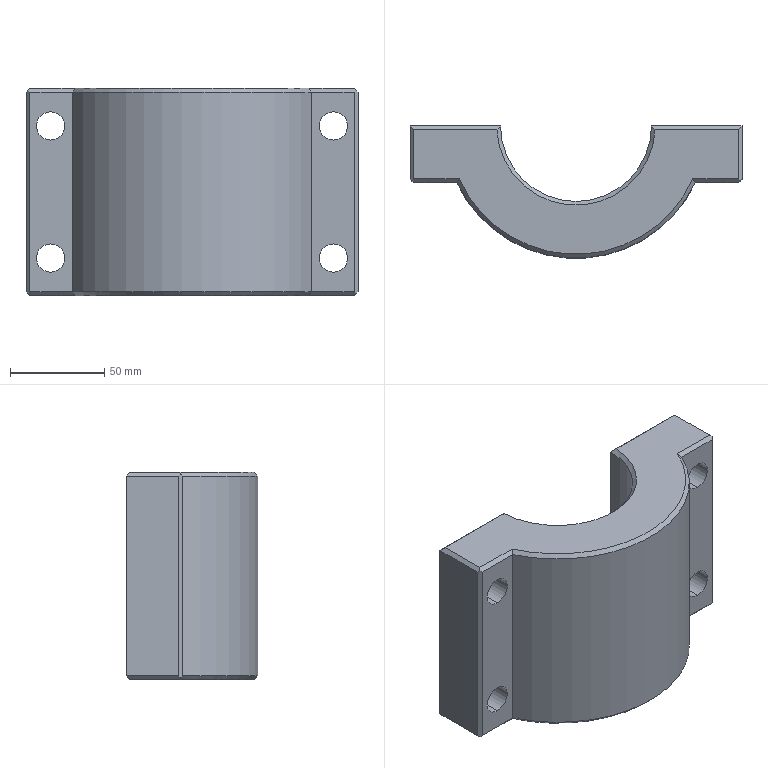Part | Creo | features DATUM PLANE 3, CURVE 2, CHAMFER 1, COORDINATE SYSTEM 1, CUT 1, PROTRUSION 1 | 1 solid | 36 faces | box 175.991 x 70 x 110 mm | volume 679965 mm3 | plane 22 | cylinder 10 | cone 4 | commonest cylinder face diameters 15 x8 80 x1 140 x1
STEP:
#1=CARTESIAN_POINT('',(0.,0.,0.));
#2=DIRECTION('',(0.,0.,1.));
#3=DIRECTION('',(1.,0.,0.));
#4=AXIS2_PLACEMENT_3D('',#1,#2,#3);
#5=CARTESIAN_POINT('',(85.991,28.,-55.));
#6=VERTEX_POINT('',#5);
#7=CARTESIAN_POINT('',(85.991,2.,-55.));
#8=VERTEX_POINT('',#7);
#9=CARTESIAN_POINT('',(85.991,28.,-55.));
#10=DIRECTION('',(0.,-1.,0.));
#11=VECTOR('',#10,26.);
#12=LINE('',#9,#11);
#13=EDGE_CURVE('',#6,#8,#12,.T.);
#14=ORIENTED_EDGE('',*,*,#13,.F.);
#15=CARTESIAN_POINT('',(41.948,28.,-55.));
#16=VERTEX_POINT('',#15);
#17=CARTESIAN_POINT('',(41.948,28.,-55.));
#18=DIRECTION('',(1.,0.,0.));
#19=VECTOR('',#18,44.043);
#20=LINE('',#17,#19);
#21=EDGE_CURVE('',#16,#6,#20,.T.);
#22=ORIENTED_EDGE('',*,*,#21,.F.);
#23=CARTESIAN_POINT('',(-41.957,28.,-55.));
#24=VERTEX_POINT('',#23);
#25=CARTESIAN_POINT('',(-0.004447,30.,-55.));
#26=DIRECTION('',(0.,0.,1.));
#27=DIRECTION('',(-0.9989,-0.04762,0.));
#28=AXIS2_PLACEMENT_3D('',#25,#26,#27);
#29=CIRCLE('',#28,42.);
#30=EDGE_CURVE('',#24,#16,#29,.T.);
#31=ORIENTED_EDGE('',*,*,#30,.F.);
#32=CARTESIAN_POINT('',(-86.,28.,-55.));
#33=VERTEX_POINT('',#32);
#34=CARTESIAN_POINT('',(-86.,28.,-55.));
#35=DIRECTION('',(1.,0.,0.));
#36=VECTOR('',#35,44.043);
#37=LINE('',#34,#36);
#38=EDGE_CURVE('',#33,#24,#37,.T.);
#39=ORIENTED_EDGE('',*,*,#38,.F.);
#40=CARTESIAN_POINT('',(-86.,2.,-55.));
#41=VERTEX_POINT('',#40);
#42=CARTESIAN_POINT('',(-86.,2.,-55.));
#43=DIRECTION('',(0.,1.,0.));
#44=VECTOR('',#43,26.);
#45=LINE('',#42,#44);
#46=EDGE_CURVE('',#41,#33,#45,.T.);
#47=ORIENTED_EDGE('',*,*,#46,.F.);
#48=CARTESIAN_POINT('',(-61.972,2.,-55.));
#49=VERTEX_POINT('',#48);
#50=CARTESIAN_POINT('',(-61.972,2.,-55.));
#51=DIRECTION('',(-1.,0.000000288,0.00000094));
#52=VECTOR('',#51,24.028);
#53=LINE('',#50,#52);
#54=EDGE_CURVE('',#49,#41,#53,.T.);
#55=ORIENTED_EDGE('',*,*,#54,.F.);
#56=CARTESIAN_POINT('',(61.963,2.,-55.));
#57=VERTEX_POINT('',#56);
#58=CARTESIAN_POINT('',(-0.004227,30.,-55.));
#59=DIRECTION('',(0.,0.,-1.));
#60=DIRECTION('',(0.9113,-0.4118,0.));
#61=AXIS2_PLACEMENT_3D('',#58,#59,#60);
#62=CIRCLE('',#61,68.);
#63=EDGE_CURVE('',#57,#49,#62,.T.);
#64=ORIENTED_EDGE('',*,*,#63,.F.);
#65=CARTESIAN_POINT('',(85.991,2.,-55.));
#66=DIRECTION('',(-1.,-0.000000343,-0.000000834));
#67=VECTOR('',#66,24.028);
#68=LINE('',#65,#67);
#69=EDGE_CURVE('',#8,#57,#68,.T.);
#70=ORIENTED_EDGE('',*,*,#69,.F.);
#71=EDGE_LOOP('',(#14,#22,#31,#39,#47,#55,#64,#70));
#72=FACE_OUTER_BOUND('',#71,.F.);
#73=CARTESIAN_POINT('',(0.,0.,-55.));
#74=DIRECTION('',(0.,0.,1.));
#75=DIRECTION('',(1.,0.,0.));
#76=AXIS2_PLACEMENT_3D('',#73,#74,#75);
#77=PLANE('',#76);
#78=ADVANCED_FACE('',(#72),#77,.F.);
#79=CARTESIAN_POINT('',(87.991,30.,-53.));
#80=VERTEX_POINT('',#79);
#81=CARTESIAN_POINT('',(87.991,2.,-53.));
#82=VERTEX_POINT('',#81);
#83=CARTESIAN_POINT('',(87.991,30.,-53.));
#84=DIRECTION('',(0.,-1.,0.));
#85=VECTOR('',#84,28.);
#86=LINE('',#83,#85);
#87=EDGE_CURVE('',#80,#82,#86,.T.);
#88=ORIENTED_EDGE('',*,*,#87,.F.);
#89=CARTESIAN_POINT('',(85.991,28.,-55.));
#90=DIRECTION('',(0.5774,0.5774,0.5774));
#91=VECTOR('',#90,3.464);
#92=LINE('',#89,#91);
#93=EDGE_CURVE('',#6,#80,#92,.T.);
#94=ORIENTED_EDGE('',*,*,#93,.F.);
#95=ORIENTED_EDGE('',*,*,#13,.T.);
#96=CARTESIAN_POINT('',(86.991,1.,-54.));
#97=VERTEX_POINT('',#96);
#98=CARTESIAN_POINT('',(86.991,1.,-54.));
#99=DIRECTION('',(-0.5774,0.5774,-0.5774));
#100=VECTOR('',#99,1.732);
#101=LINE('',#98,#100);
#102=EDGE_CURVE('',#97,#8,#101,.T.);
#103=ORIENTED_EDGE('',*,*,#102,.F.);
#104=CARTESIAN_POINT('',(87.991,2.,-53.));
#105=DIRECTION('',(-0.5774,-0.5774,-0.5774));
#106=VECTOR('',#105,1.732);
#107=LINE('',#104,#106);
#108=EDGE_CURVE('',#82,#97,#107,.T.);
#109=ORIENTED_EDGE('',*,*,#108,.F.);
#110=EDGE_LOOP('',(#88,#94,#95,#103,#109));
#111=FACE_OUTER_BOUND('',#110,.F.);
#112=CARTESIAN_POINT('',(86.991,15.,-54.));
#113=DIRECTION('',(0.7071,0.,-0.7071));
#114=DIRECTION('',(0.7071,0.,0.7071));
#115=AXIS2_PLACEMENT_3D('',#112,#113,#114);
#116=PLANE('',#115);
#117=ADVANCED_FACE('',(#111),#116,.T.);
#118=CARTESIAN_POINT('',(87.991,2.,53.));
#119=VERTEX_POINT('',#118);
#120=CARTESIAN_POINT('',(87.991,30.,53.));
#121=VERTEX_POINT('',#120);
#122=CARTESIAN_POINT('',(87.991,2.,53.));
#123=DIRECTION('',(0.,1.,0.));
#124=VECTOR('',#123,28.);
#125=LINE('',#122,#124);
#126=EDGE_CURVE('',#119,#121,#125,.T.);
#127=ORIENTED_EDGE('',*,*,#126,.T.);
#128=CARTESIAN_POINT('',(87.991,30.,-53.));
#129=DIRECTION('',(0.,0.,1.));
#130=VECTOR('',#129,106.);
#131=LINE('',#128,#130);
#132=EDGE_CURVE('',#80,#121,#131,.T.);
#133=ORIENTED_EDGE('',*,*,#132,.F.);
#134=ORIENTED_EDGE('',*,*,#87,.T.);
#135=CARTESIAN_POINT('',(87.991,2.,53.));
#136=DIRECTION('',(0.,0.,-1.));
#137=VECTOR('',#136,106.);
#138=LINE('',#135,#137);
#139=EDGE_CURVE('',#119,#82,#138,.T.);
#140=ORIENTED_EDGE('',*,*,#139,.F.);
#141=EDGE_LOOP('',(#127,#133,#134,#140));
#142=FACE_OUTER_BOUND('',#141,.F.);
#143=CARTESIAN_POINT('',(87.991,0.,-55.));
#144=DIRECTION('',(1.,0.,0.));
#145=DIRECTION('',(0.,1.,0.));
#146=AXIS2_PLACEMENT_3D('',#143,#144,#145);
#147=PLANE('',#146);
#148=ADVANCED_FACE('',(#142),#147,.T.);
#149=CARTESIAN_POINT('',(85.991,2.,55.));
#150=VERTEX_POINT('',#149);
#151=CARTESIAN_POINT('',(85.991,28.,55.));
#152=VERTEX_POINT('',#151);
#153=CARTESIAN_POINT('',(85.991,2.,55.));
#154=DIRECTION('',(0.,1.,0.));
#155=VECTOR('',#154,26.);
#156=LINE('',#153,#155);
#157=EDGE_CURVE('',#150,#152,#156,.T.);
#158=ORIENTED_EDGE('',*,*,#157,.T.);
#159=CARTESIAN_POINT('',(87.991,30.,53.));
#160=DIRECTION('',(-0.5774,-0.5774,0.5774));
#161=VECTOR('',#160,3.464);
#162=LINE('',#159,#161);
#163=EDGE_CURVE('',#121,#152,#162,.T.);
#164=ORIENTED_EDGE('',*,*,#163,.F.);
#165=ORIENTED_EDGE('',*,*,#126,.F.);
#166=CARTESIAN_POINT('',(86.991,1.,54.));
#167=VERTEX_POINT('',#166);
#168=CARTESIAN_POINT('',(87.991,2.,53.));
#169=DIRECTION('',(-0.5774,-0.5774,0.5774));
#170=VECTOR('',#169,1.732);
#171=LINE('',#168,#170);
#172=EDGE_CURVE('',#119,#167,#171,.T.);
#173=ORIENTED_EDGE('',*,*,#172,.T.);
#174=CARTESIAN_POINT('',(85.991,2.,55.));
#175=DIRECTION('',(0.5774,-0.5774,-0.5774));
#176=VECTOR('',#175,1.732);
#177=LINE('',#174,#176);
#178=EDGE_CURVE('',#150,#167,#177,.T.);
#179=ORIENTED_EDGE('',*,*,#178,.F.);
#180=EDGE_LOOP('',(#158,#164,#165,#173,#179));
#181=FACE_OUTER_BOUND('',#180,.F.);
#182=CARTESIAN_POINT('',(86.991,15.,54.));
#183=DIRECTION('',(0.7071,0.,0.7071));
#184=DIRECTION('',(0.7071,0.,-0.7071));
#185=AXIS2_PLACEMENT_3D('',#182,#183,#184);
#186=PLANE('',#185);
#187=ADVANCED_FACE('',(#181),#186,.T.);
#188=CARTESIAN_POINT('',(61.963,2.,55.));
#189=VERTEX_POINT('',#188);
#190=CARTESIAN_POINT('',(61.963,2.,55.));
#191=DIRECTION('',(1.,0.000000404,-0.000000742));
#192=VECTOR('',#191,24.028);
#193=LINE('',#190,#192);
#194=EDGE_CURVE('',#189,#150,#193,.T.);
#195=ORIENTED_EDGE('',*,*,#194,.F.);
#196=CARTESIAN_POINT('',(-61.972,2.,55.));
#197=VERTEX_POINT('',#196);
#198=CARTESIAN_POINT('',(-0.004674,30.,55.));
#199=DIRECTION('',(0.,0.,1.));
#200=DIRECTION('',(-0.9113,-0.4118,0.));
#201=AXIS2_PLACEMENT_3D('',#198,#199,#200);
#202=CIRCLE('',#201,68.);
#203=EDGE_CURVE('',#197,#189,#202,.T.);
#204=ORIENTED_EDGE('',*,*,#203,.F.);
#205=CARTESIAN_POINT('',(-86.,2.,55.));
#206=VERTEX_POINT('',#205);
#207=CARTESIAN_POINT('',(-86.,2.,55.));
#208=DIRECTION('',(1.,-0.000000349,0.000000849));
#209=VECTOR('',#208,24.028);
#210=LINE('',#207,#209);
#211=EDGE_CURVE('',#206,#197,#210,.T.);
#212=ORIENTED_EDGE('',*,*,#211,.F.);
#213=CARTESIAN_POINT('',(-86.,28.,55.));
#214=VERTEX_POINT('',#213);
#215=CARTESIAN_POINT('',(-86.,28.,55.));
#216=DIRECTION('',(0.,-1.,0.));
#217=VECTOR('',#216,26.);
#218=LINE('',#215,#217);
#219=EDGE_CURVE('',#214,#206,#218,.T.);
#220=ORIENTED_EDGE('',*,*,#219,.F.);
#221=CARTESIAN_POINT('',(-41.957,28.,55.));
#222=VERTEX_POINT('',#221);
#223=CARTESIAN_POINT('',(-41.957,28.,55.));
#224=DIRECTION('',(-1.,0.,0.));
#225=VECTOR('',#224,44.043);
#226=LINE('',#223,#225);
#227=EDGE_CURVE('',#222,#214,#226,.T.);
#228=ORIENTED_EDGE('',*,*,#227,.F.);
#229=CARTESIAN_POINT('',(41.948,28.,55.));
#230=VERTEX_POINT('',#229);
#231=CARTESIAN_POINT('',(-0.004447,30.,55.));
#232=DIRECTION('',(0.,0.,-1.));
#233=DIRECTION('',(0.9989,-0.04762,0.));
#234=AXIS2_PLACEMENT_3D('',#231,#232,#233);
#235=CIRCLE('',#234,42.);
#236=EDGE_CURVE('',#230,#222,#235,.T.);
#237=ORIENTED_EDGE('',*,*,#236,.F.);
#238=CARTESIAN_POINT('',(85.991,28.,55.));
#239=DIRECTION('',(-1.,0.,0.));
#240=VECTOR('',#239,44.043);
#241=LINE('',#238,#240);
#242=EDGE_CURVE('',#152,#230,#241,.T.);
#243=ORIENTED_EDGE('',*,*,#242,.F.);
#244=ORIENTED_EDGE('',*,*,#157,.F.);
#245=EDGE_LOOP('',(#195,#204,#212,#220,#228,#237,#243,#244));
#246=FACE_OUTER_BOUND('',#245,.F.);
#247=CARTESIAN_POINT('',(0.,0.,55.));
#248=DIRECTION('',(0.,0.,1.));
#249=DIRECTION('',(1.,0.,0.));
#250=AXIS2_PLACEMENT_3D('',#247,#248,#249);
#251=PLANE('',#250);
#252=ADVANCED_FACE('',(#246),#251,.T.);
#253=CARTESIAN_POINT('',(63.241,-0.000008615,53.));
#254=VERTEX_POINT('',#253);
#255=CARTESIAN_POINT('',(85.991,0.,53.));
#256=VERTEX_POINT('',#255);
#257=CARTESIAN_POINT('',(63.241,-0.000008615,53.));
#258=DIRECTION('',(1.,0.000000379,-0.000000698));
#259=VECTOR('',#258,22.75);
#260=LINE('',#257,#259);
#261=EDGE_CURVE('',#254,#256,#260,.T.);
#262=ORIENTED_EDGE('',*,*,#261,.F.);
#263=CARTESIAN_POINT('',(63.241,-0.000008615,53.));
#264=CARTESIAN_POINT('',(63.098,0.2256,53.226));
#265=CARTESIAN_POINT('',(62.814,0.6747,53.675));
#266=CARTESIAN_POINT('',(62.388,1.341,54.341));
#267=CARTESIAN_POINT('',(62.104,1.781,54.781));
#268=CARTESIAN_POINT('',(61.963,2.,55.));
#269=B_SPLINE_CURVE_WITH_KNOTS('',3,(#263,#264,#265,#266,#267,#268),.UNSPECIFIED.,.F.,.F.,(4,1,1,4),(0.,0.3333,0.6667,1.),.UNSPECIFIED.);
#270=EDGE_CURVE('',#254,#189,#269,.T.);
#271=ORIENTED_EDGE('',*,*,#270,.T.);
#272=ORIENTED_EDGE('',*,*,#194,.T.);
#273=ORIENTED_EDGE('',*,*,#178,.T.);
#274=CARTESIAN_POINT('',(86.991,1.,54.));
#275=DIRECTION('',(-0.5774,-0.5774,-0.5774));
#276=VECTOR('',#275,1.732);
#277=LINE('',#274,#276);
#278=EDGE_CURVE('',#167,#256,#277,.T.);
#279=ORIENTED_EDGE('',*,*,#278,.T.);
#280=EDGE_LOOP('',(#262,#271,#272,#273,#279));
#281=FACE_OUTER_BOUND('',#280,.F.);
#282=CARTESIAN_POINT('',(75.616,1.,54.));
#283=DIRECTION('',(0.,-0.7071,0.7071));
#284=DIRECTION('',(0.,-0.7071,-0.7071));
#285=AXIS2_PLACEMENT_3D('',#282,#283,#284);
#286=PLANE('',#285);
#287=ADVANCED_FACE('',(#281),#286,.T.);
#288=ORIENTED_EDGE('',*,*,#261,.T.);
#289=CARTESIAN_POINT('',(85.991,0.,-53.));
#290=VERTEX_POINT('',#289);
#291=CARTESIAN_POINT('',(85.991,0.,53.));
#292=DIRECTION('',(0.,0.,-1.));
#293=VECTOR('',#292,106.);
#294=LINE('',#291,#293);
#295=EDGE_CURVE('',#256,#290,#294,.T.);
#296=ORIENTED_EDGE('',*,*,#295,.T.);
#297=CARTESIAN_POINT('',(63.241,-0.000007516,-53.));
#298=VERTEX_POINT('',#297);
#299=CARTESIAN_POINT('',(85.991,0.,-53.));
#300=DIRECTION('',(-1.,-0.00000033,-0.000000771));
#301=VECTOR('',#300,22.75);
#302=LINE('',#299,#301);
#303=EDGE_CURVE('',#290,#298,#302,.T.);
#304=ORIENTED_EDGE('',*,*,#303,.T.);
#305=CARTESIAN_POINT('',(63.241,-0.000007516,-53.));
#306=DIRECTION('',(-0.000001055,-0.00000001,1.));
#307=VECTOR('',#306,106.);
#308=LINE('',#305,#307);
#309=EDGE_CURVE('',#298,#254,#308,.T.);
#310=ORIENTED_EDGE('',*,*,#309,.T.);
#311=EDGE_LOOP('',(#288,#296,#304,#310));
#312=FACE_OUTER_BOUND('',#311,.F.);
#313=CARTESIAN_POINT('',(75.,0.,27.5));
#314=VERTEX_POINT('',#313);
#315=CARTESIAN_POINT('',(75.,0.,42.5));
#316=VERTEX_POINT('',#315);
#317=CARTESIAN_POINT('',(75.,0.,35.));
#318=DIRECTION('',(0.,-1.,0.));
#319=DIRECTION('',(0.,0.,-1.));
#320=AXIS2_PLACEMENT_3D('',#317,#318,#319);
#321=CIRCLE('',#320,7.5);
#322=EDGE_CURVE('',#314,#316,#321,.T.);
#323=ORIENTED_EDGE('',*,*,#322,.T.);
#324=CARTESIAN_POINT('',(75.,0.,35.));
#325=DIRECTION('',(0.,-1.,0.));
#326=DIRECTION('',(0.,0.,1.));
#327=AXIS2_PLACEMENT_3D('',#324,#325,#326);
#328=CIRCLE('',#327,7.5);
#329=EDGE_CURVE('',#316,#314,#328,.T.);
#330=ORIENTED_EDGE('',*,*,#329,.T.);
#331=EDGE_LOOP('',(#323,#330));
#332=FACE_BOUND('',#331,.F.);
#333=CARTESIAN_POINT('',(75.,0.,-42.5));
#334=VERTEX_POINT('',#333);
#335=CARTESIAN_POINT('',(75.,0.,-27.5));
#336=VERTEX_POINT('',#335);
#337=CARTESIAN_POINT('',(75.,0.,-35.));
#338=DIRECTION('',(0.,-1.,0.));
#339=DIRECTION('',(0.,0.,-1.));
#340=AXIS2_PLACEMENT_3D('',#337,#338,#339);
#341=CIRCLE('',#340,7.5);
#342=EDGE_CURVE('',#334,#336,#341,.T.);
#343=ORIENTED_EDGE('',*,*,#342,.T.);
#344=CARTESIAN_POINT('',(75.,0.,-35.));
#345=DIRECTION('',(0.,-1.,0.));
#346=DIRECTION('',(0.,0.,1.));
#347=AXIS2_PLACEMENT_3D('',#344,#345,#346);
#348=CIRCLE('',#347,7.5);
#349=EDGE_CURVE('',#336,#334,#348,.T.);
#350=ORIENTED_EDGE('',*,*,#349,.T.);
#351=EDGE_LOOP('',(#343,#350));
#352=FACE_BOUND('',#351,.F.);
#353=CARTESIAN_POINT('',(63.241,0.,-55.));
#354=DIRECTION('',(0.,-1.,0.));
#355=DIRECTION('',(1.,0.,0.));
#356=AXIS2_PLACEMENT_3D('',#353,#354,#355);
#357=PLANE('',#356);
#358=ADVANCED_FACE('',(#312,#332,#352),#357,.T.);
#359=CARTESIAN_POINT('',(75.,30.,-42.5));
#360=VERTEX_POINT('',#359);
#361=CARTESIAN_POINT('',(75.,30.,-27.5));
#362=VERTEX_POINT('',#361);
#363=CARTESIAN_POINT('',(75.,30.,-35.));
#364=DIRECTION('',(0.,-1.,0.));
#365=DIRECTION('',(0.,0.,-1.));
#366=AXIS2_PLACEMENT_3D('',#363,#364,#365);
#367=CIRCLE('',#366,7.5);
#368=EDGE_CURVE('',#360,#362,#367,.T.);
#369=ORIENTED_EDGE('',*,*,#368,.T.);
#370=CARTESIAN_POINT('',(75.,0.,-27.5));
#371=DIRECTION('',(0.,1.,0.));
#372=VECTOR('',#371,30.);
#373=LINE('',#370,#372);
#374=EDGE_CURVE('',#336,#362,#373,.T.);
#375=ORIENTED_EDGE('',*,*,#374,.F.);
#376=ORIENTED_EDGE('',*,*,#342,.F.);
#377=CARTESIAN_POINT('',(75.,0.,-42.5));
#378=DIRECTION('',(0.,1.,0.));
#379=VECTOR('',#378,30.);
#380=LINE('',#377,#379);
#381=EDGE_CURVE('',#334,#360,#380,.T.);
#382=ORIENTED_EDGE('',*,*,#381,.T.);
#383=EDGE_LOOP('',(#369,#375,#376,#382));
#384=FACE_OUTER_BOUND('',#383,.F.);
#385=CARTESIAN_POINT('',(75.,0.,-35.));
#386=DIRECTION('',(0.,-1.,0.));
#387=DIRECTION('',(0.,0.,-1.));
#388=AXIS2_PLACEMENT_3D('',#385,#386,#387);
#389=CYLINDRICAL_SURFACE('',#388,7.5);
#390=ADVANCED_FACE('',(#384),#389,.F.);
#391=CARTESIAN_POINT('',(39.996,30.,53.));
#392=VERTEX_POINT('',#391);
#393=CARTESIAN_POINT('',(87.991,30.,53.));
#394=DIRECTION('',(-1.,0.,0.));
#395=VECTOR('',#394,47.996);
#396=LINE('',#393,#395);
#397=EDGE_CURVE('',#121,#392,#396,.T.);
#398=ORIENTED_EDGE('',*,*,#397,.T.);
#399=CARTESIAN_POINT('',(39.996,30.,-53.));
#400=VERTEX_POINT('',#399);
#401=CARTESIAN_POINT('',(39.996,30.,-53.));
#402=DIRECTION('',(0.,0.,1.));
#403=VECTOR('',#402,106.);
#404=LINE('',#401,#403);
#405=EDGE_CURVE('',#400,#392,#404,.T.);
#406=ORIENTED_EDGE('',*,*,#405,.F.);
#407=CARTESIAN_POINT('',(39.996,30.,-53.));
#408=DIRECTION('',(1.,0.,0.));
#409=VECTOR('',#408,47.996);
#410=LINE('',#407,#409);
#411=EDGE_CURVE('',#400,#80,#410,.T.);
#412=ORIENTED_EDGE('',*,*,#411,.T.);
#413=ORIENTED_EDGE('',*,*,#132,.T.);
#414=EDGE_LOOP('',(#398,#406,#412,#413));
#415=FACE_OUTER_BOUND('',#414,.F.);
#416=CARTESIAN_POINT('',(75.,30.,27.5));
#417=VERTEX_POINT('',#416);
#418=CARTESIAN_POINT('',(75.,30.,42.5));
#419=VERTEX_POINT('',#418);
#420=CARTESIAN_POINT('',(75.,30.,35.));
#421=DIRECTION('',(0.,-1.,0.));
#422=DIRECTION('',(0.,0.,-1.));
#423=AXIS2_PLACEMENT_3D('',#420,#421,#422);
#424=CIRCLE('',#423,7.5);
#425=EDGE_CURVE('',#417,#419,#424,.T.);
#426=ORIENTED_EDGE('',*,*,#425,.F.);
#427=CARTESIAN_POINT('',(75.,30.,35.));
#428=DIRECTION('',(0.,-1.,0.));
#429=DIRECTION('',(0.,0.,1.));
#430=AXIS2_PLACEMENT_3D('',#427,#428,#429);
#431=CIRCLE('',#430,7.5);
#432=EDGE_CURVE('',#419,#417,#431,.T.);
#433=ORIENTED_EDGE('',*,*,#432,.F.);
#434=EDGE_LOOP('',(#426,#433));
#435=FACE_BOUND('',#434,.F.);
#436=ORIENTED_EDGE('',*,*,#368,.F.);
#437=CARTESIAN_POINT('',(75.,30.,-35.));
#438=DIRECTION('',(0.,-1.,0.));
#439=DIRECTION('',(0.,0.,1.));
#440=AXIS2_PLACEMENT_3D('',#437,#438,#439);
#441=CIRCLE('',#440,7.5);
#442=EDGE_CURVE('',#362,#360,#441,.T.);
#443=ORIENTED_EDGE('',*,*,#442,.F.);
#444=EDGE_LOOP('',(#436,#443));
#445=FACE_BOUND('',#444,.F.);
#446=CARTESIAN_POINT('',(87.991,30.,-55.));
#447=DIRECTION('',(0.,1.,0.));
#448=DIRECTION('',(-1.,0.,0.));
#449=AXIS2_PLACEMENT_3D('',#446,#447,#448);
#450=PLANE('',#449);
#451=ADVANCED_FACE('',(#415,#435,#445),#450,.T.);
#452=ORIENTED_EDGE('',*,*,#442,.T.);
#453=ORIENTED_EDGE('',*,*,#381,.F.);
#454=ORIENTED_EDGE('',*,*,#349,.F.);
#455=ORIENTED_EDGE('',*,*,#374,.T.);
#456=EDGE_LOOP('',(#452,#453,#454,#455));
#457=FACE_OUTER_BOUND('',#456,.F.);
#458=CARTESIAN_POINT('',(75.,0.,-35.));
#459=DIRECTION('',(0.,-1.,0.));
#460=DIRECTION('',(0.,0.,-1.));
#461=AXIS2_PLACEMENT_3D('',#458,#459,#460);
#462=CYLINDRICAL_SURFACE('',#461,7.5);
#463=ADVANCED_FACE('',(#457),#462,.F.);
#464=ORIENTED_EDGE('',*,*,#425,.T.);
#465=CARTESIAN_POINT('',(75.,0.,42.5));
#466=DIRECTION('',(0.,1.,0.));
#467=VECTOR('',#466,30.);
#468=LINE('',#465,#467);
#469=EDGE_CURVE('',#316,#419,#468,.T.);
#470=ORIENTED_EDGE('',*,*,#469,.F.);
#471=ORIENTED_EDGE('',*,*,#322,.F.);
#472=CARTESIAN_POINT('',(75.,0.,27.5));
#473=DIRECTION('',(0.,1.,0.));
#474=VECTOR('',#473,30.);
#475=LINE('',#472,#474);
#476=EDGE_CURVE('',#314,#417,#475,.T.);
#477=ORIENTED_EDGE('',*,*,#476,.T.);
#478=EDGE_LOOP('',(#464,#470,#471,#477));
#479=FACE_OUTER_BOUND('',#478,.F.);
#480=CARTESIAN_POINT('',(75.,0.,35.));
#481=DIRECTION('',(0.,-1.,0.));
#482=DIRECTION('',(0.,0.,-1.));
#483=AXIS2_PLACEMENT_3D('',#480,#481,#482);
#484=CYLINDRICAL_SURFACE('',#483,7.5);
#485=ADVANCED_FACE('',(#479),#484,.F.);
#486=ORIENTED_EDGE('',*,*,#432,.T.);
#487=ORIENTED_EDGE('',*,*,#476,.F.);
#488=ORIENTED_EDGE('',*,*,#329,.F.);
#489=ORIENTED_EDGE('',*,*,#469,.T.);
#490=EDGE_LOOP('',(#486,#487,#488,#489));
#491=FACE_OUTER_BOUND('',#490,.F.);
#492=CARTESIAN_POINT('',(75.,0.,35.));
#493=DIRECTION('',(0.,-1.,0.));
#494=DIRECTION('',(0.,0.,-1.));
#495=AXIS2_PLACEMENT_3D('',#492,#493,#494);
#496=CYLINDRICAL_SURFACE('',#495,7.5);
#497=ADVANCED_FACE('',(#491),#496,.F.);
#498=ORIENTED_EDGE('',*,*,#397,.F.);
#499=ORIENTED_EDGE('',*,*,#163,.T.);
#500=ORIENTED_EDGE('',*,*,#242,.T.);
#501=CARTESIAN_POINT('',(39.996,30.,53.));
#502=CARTESIAN_POINT('',(40.211,29.785,53.215));
#503=CARTESIAN_POINT('',(40.642,29.35,53.65));
#504=CARTESIAN_POINT('',(41.293,28.683,54.317));
#505=CARTESIAN_POINT('',(41.729,28.229,54.771));
#506=CARTESIAN_POINT('',(41.948,28.,55.));
#507=B_SPLINE_CURVE_WITH_KNOTS('',3,(#501,#502,#503,#504,#505,#506),.UNSPECIFIED.,.F.,.F.,(4,1,1,4),(0.,0.3333,0.6667,1.),.UNSPECIFIED.);
#508=EDGE_CURVE('',#392,#230,#507,.T.);
#509=ORIENTED_EDGE('',*,*,#508,.F.);
#510=EDGE_LOOP('',(#498,#499,#500,#509));
#511=FACE_OUTER_BOUND('',#510,.F.);
#512=CARTESIAN_POINT('',(63.993,29.,54.));
#513=DIRECTION('',(0.,0.7071,0.7071));
#514=DIRECTION('',(0.,0.7071,-0.7071));
#515=AXIS2_PLACEMENT_3D('',#512,#513,#514);
#516=PLANE('',#515);
#517=ADVANCED_FACE('',(#511),#516,.T.);
#518=ORIENTED_EDGE('',*,*,#236,.T.);
#519=CARTESIAN_POINT('',(-40.004,30.,53.));
#520=VERTEX_POINT('',#519);
#521=CARTESIAN_POINT('',(-40.004,30.,53.));
#522=CARTESIAN_POINT('',(-40.22,29.785,53.215));
#523=CARTESIAN_POINT('',(-40.651,29.35,53.65));
#524=CARTESIAN_POINT('',(-41.302,28.683,54.317));
#525=CARTESIAN_POINT('',(-41.738,28.229,54.771));
#526=CARTESIAN_POINT('',(-41.957,28.,55.));
#527=B_SPLINE_CURVE_WITH_KNOTS('',3,(#521,#522,#523,#524,#525,#526),.UNSPECIFIED.,.F.,.F.,(4,1,1,4),(0.,0.3333,0.6667,1.),.UNSPECIFIED.);
#528=EDGE_CURVE('',#520,#222,#527,.T.);
#529=ORIENTED_EDGE('',*,*,#528,.F.);
#530=CARTESIAN_POINT('',(-0.004447,30.,53.));
#531=DIRECTION('',(0.,0.,1.));
#532=DIRECTION('',(-1.,0.,0.));
#533=AXIS2_PLACEMENT_3D('',#530,#531,#532);
#534=CIRCLE('',#533,40.);
#535=EDGE_CURVE('',#520,#392,#534,.T.);
#536=ORIENTED_EDGE('',*,*,#535,.T.);
#537=ORIENTED_EDGE('',*,*,#508,.T.);
#538=EDGE_LOOP('',(#518,#529,#536,#537));
#539=FACE_OUTER_BOUND('',#538,.F.);
#540=CARTESIAN_POINT('',(-0.004447,30.,54.));
#541=DIRECTION('',(0.,0.,1.));
#542=DIRECTION('',(0.,-1.,0.));
#543=AXIS2_PLACEMENT_3D('',#540,#541,#542);
#544=CONICAL_SURFACE('',#543,41.,45.);
#545=ADVANCED_FACE('',(#539),#544,.F.);
#546=CARTESIAN_POINT('',(-88.,30.,53.));
#547=VERTEX_POINT('',#546);
#548=CARTESIAN_POINT('',(-40.004,30.,53.));
#549=DIRECTION('',(-1.,0.,0.));
#550=VECTOR('',#549,47.996);
#551=LINE('',#548,#550);
#552=EDGE_CURVE('',#520,#547,#551,.T.);
#553=ORIENTED_EDGE('',*,*,#552,.F.);
#554=ORIENTED_EDGE('',*,*,#528,.T.);
#555=ORIENTED_EDGE('',*,*,#227,.T.);
#556=CARTESIAN_POINT('',(-88.,30.,53.));
#557=DIRECTION('',(0.5774,-0.5774,0.5774));
#558=VECTOR('',#557,3.464);
#559=LINE('',#556,#558);
#560=EDGE_CURVE('',#547,#214,#559,.T.);
#561=ORIENTED_EDGE('',*,*,#560,.F.);
#562=EDGE_LOOP('',(#553,#554,#555,#561));
#563=FACE_OUTER_BOUND('',#562,.F.);
#564=CARTESIAN_POINT('',(-64.002,29.,54.));
#565=DIRECTION('',(0.,0.7071,0.7071));
#566=DIRECTION('',(0.,0.7071,-0.7071));
#567=AXIS2_PLACEMENT_3D('',#564,#565,#566);
#568=PLANE('',#567);
#569=ADVANCED_FACE('',(#563),#568,.T.);
#570=ORIENTED_EDGE('',*,*,#552,.T.);
#571=CARTESIAN_POINT('',(-88.,30.,-53.));
#572=VERTEX_POINT('',#571);
#573=CARTESIAN_POINT('',(-88.,30.,-53.));
#574=DIRECTION('',(0.,0.,1.));
#575=VECTOR('',#574,106.);
#576=LINE('',#573,#575);
#577=EDGE_CURVE('',#572,#547,#576,.T.);
#578=ORIENTED_EDGE('',*,*,#577,.F.);
#579=CARTESIAN_POINT('',(-40.004,30.,-53.));
#580=VERTEX_POINT('',#579);
#581=CARTESIAN_POINT('',(-88.,30.,-53.));
#582=DIRECTION('',(1.,0.,0.));
#583=VECTOR('',#582,47.996);
#584=LINE('',#581,#583);
#585=EDGE_CURVE('',#572,#580,#584,.T.);
#586=ORIENTED_EDGE('',*,*,#585,.T.);
#587=CARTESIAN_POINT('',(-40.004,30.,-53.));
#588=DIRECTION('',(0.,0.,1.));
#589=VECTOR('',#588,106.);
#590=LINE('',#587,#589);
#591=EDGE_CURVE('',#580,#520,#590,.T.);
#592=ORIENTED_EDGE('',*,*,#591,.T.);
#593=EDGE_LOOP('',(#570,#578,#586,#592));
#594=FACE_OUTER_BOUND('',#593,.F.);
#595=CARTESIAN_POINT('',(-75.,30.,27.5));
#596=VERTEX_POINT('',#595);
#597=CARTESIAN_POINT('',(-75.,30.,42.5));
#598=VERTEX_POINT('',#597);
#599=CARTESIAN_POINT('',(-75.,30.,35.));
#600=DIRECTION('',(0.,-1.,0.));
#601=DIRECTION('',(0.,0.,-1.));
#602=AXIS2_PLACEMENT_3D('',#599,#600,#601);
#603=CIRCLE('',#602,7.5);
#604=EDGE_CURVE('',#596,#598,#603,.T.);
#605=ORIENTED_EDGE('',*,*,#604,.F.);
#606=CARTESIAN_POINT('',(-75.,30.,35.));
#607=DIRECTION('',(0.,-1.,0.));
#608=DIRECTION('',(0.,0.,1.));
#609=AXIS2_PLACEMENT_3D('',#606,#607,#608);
#610=CIRCLE('',#609,7.5);
#611=EDGE_CURVE('',#598,#596,#610,.T.);
#612=ORIENTED_EDGE('',*,*,#611,.F.);
#613=EDGE_LOOP('',(#605,#612));
#614=FACE_BOUND('',#613,.F.);
#615=CARTESIAN_POINT('',(-75.,30.,-42.5));
#616=VERTEX_POINT('',#615);
#617=CARTESIAN_POINT('',(-75.,30.,-27.5));
#618=VERTEX_POINT('',#617);
#619=CARTESIAN_POINT('',(-75.,30.,-35.));
#620=DIRECTION('',(0.,-1.,0.));
#621=DIRECTION('',(0.,0.,-1.));
#622=AXIS2_PLACEMENT_3D('',#619,#620,#621);
#623=CIRCLE('',#622,7.5);
#624=EDGE_CURVE('',#616,#618,#623,.T.);
#625=ORIENTED_EDGE('',*,*,#624,.F.);
#626=CARTESIAN_POINT('',(-75.,30.,-35.));
#627=DIRECTION('',(0.,-1.,0.));
#628=DIRECTION('',(0.,0.,1.));
#629=AXIS2_PLACEMENT_3D('',#626,#627,#628);
#630=CIRCLE('',#629,7.5);
#631=EDGE_CURVE('',#618,#616,#630,.T.);
#632=ORIENTED_EDGE('',*,*,#631,.F.);
#633=EDGE_LOOP('',(#625,#632));
#634=FACE_BOUND('',#633,.F.);
#635=CARTESIAN_POINT('',(-40.004,30.,-55.));
#636=DIRECTION('',(0.,1.,0.));
#637=DIRECTION('',(-1.,0.,0.));
#638=AXIS2_PLACEMENT_3D('',#635,#636,#637);
#639=PLANE('',#638);
#640=ADVANCED_FACE('',(#594,#614,#634),#639,.T.);
#641=ORIENTED_EDGE('',*,*,#624,.T.);
#642=CARTESIAN_POINT('',(-75.,0.,-27.5));
#643=VERTEX_POINT('',#642);
#644=CARTESIAN_POINT('',(-75.,0.,-27.5));
#645=DIRECTION('',(0.,1.,0.));
#646=VECTOR('',#645,30.);
#647=LINE('',#644,#646);
#648=EDGE_CURVE('',#643,#618,#647,.T.);
#649=ORIENTED_EDGE('',*,*,#648,.F.);
#650=CARTESIAN_POINT('',(-75.,0.,-42.5));
#651=VERTEX_POINT('',#650);
#652=CARTESIAN_POINT('',(-75.,0.,-35.));
#653=DIRECTION('',(0.,-1.,0.));
#654=DIRECTION('',(0.,0.,-1.));
#655=AXIS2_PLACEMENT_3D('',#652,#653,#654);
#656=CIRCLE('',#655,7.5);
#657=EDGE_CURVE('',#651,#643,#656,.T.);
#658=ORIENTED_EDGE('',*,*,#657,.F.);
#659=CARTESIAN_POINT('',(-75.,0.,-42.5));
#660=DIRECTION('',(0.,1.,0.));
#661=VECTOR('',#660,30.);
#662=LINE('',#659,#661);
#663=EDGE_CURVE('',#651,#616,#662,.T.);
#664=ORIENTED_EDGE('',*,*,#663,.T.);
#665=EDGE_LOOP('',(#641,#649,#658,#664));
#666=FACE_OUTER_BOUND('',#665,.F.);
#667=CARTESIAN_POINT('',(-75.,0.,-35.));
#668=DIRECTION('',(0.,-1.,0.));
#669=DIRECTION('',(0.,0.,-1.));
#670=AXIS2_PLACEMENT_3D('',#667,#668,#669);
#671=CYLINDRICAL_SURFACE('',#670,7.5);
#672=ADVANCED_FACE('',(#666),#671,.F.);
#673=ORIENTED_EDGE('',*,*,#631,.T.);
#674=ORIENTED_EDGE('',*,*,#663,.F.);
#675=CARTESIAN_POINT('',(-75.,0.,-35.));
#676=DIRECTION('',(0.,-1.,0.));
#677=DIRECTION('',(0.,0.,1.));
#678=AXIS2_PLACEMENT_3D('',#675,#676,#677);
#679=CIRCLE('',#678,7.5);
#680=EDGE_CURVE('',#643,#651,#679,.T.);
#681=ORIENTED_EDGE('',*,*,#680,.F.);
#682=ORIENTED_EDGE('',*,*,#648,.T.);
#683=EDGE_LOOP('',(#673,#674,#681,#682));
#684=FACE_OUTER_BOUND('',#683,.F.);
#685=CARTESIAN_POINT('',(-75.,0.,-35.));
#686=DIRECTION('',(0.,-1.,0.));
#687=DIRECTION('',(0.,0.,-1.));
#688=AXIS2_PLACEMENT_3D('',#685,#686,#687);
#689=CYLINDRICAL_SURFACE('',#688,7.5);
#690=ADVANCED_FACE('',(#684),#689,.F.);
#691=CARTESIAN_POINT('',(-86.,0.,53.));
#692=VERTEX_POINT('',#691);
#693=CARTESIAN_POINT('',(-63.25,-0.000007633,53.));
#694=VERTEX_POINT('',#693);
#695=CARTESIAN_POINT('',(-86.,0.,53.));
#696=DIRECTION('',(1.,-0.000000336,0.000000783));
#697=VECTOR('',#696,22.75);
#698=LINE('',#695,#697);
#699=EDGE_CURVE('',#692,#694,#698,.T.);
#700=ORIENTED_EDGE('',*,*,#699,.T.);
#701=CARTESIAN_POINT('',(-63.25,-0.000006533,-53.));
#702=VERTEX_POINT('',#701);
#703=CARTESIAN_POINT('',(-63.25,-0.000006533,-53.));
#704=DIRECTION('',(-0.000001055,-0.00000001,1.));
#705=VECTOR('',#704,106.);
#706=LINE('',#703,#705);
#707=EDGE_CURVE('',#702,#694,#706,.T.);
#708=ORIENTED_EDGE('',*,*,#707,.F.);
#709=CARTESIAN_POINT('',(-86.,0.,-53.));
#710=VERTEX_POINT('',#709);
#711=CARTESIAN_POINT('',(-63.25,-0.000006533,-53.));
#712=DIRECTION('',(-1.,0.000000287,0.000000855));
#713=VECTOR('',#712,22.75);
#714=LINE('',#711,#713);
#715=EDGE_CURVE('',#702,#710,#714,.T.);
#716=ORIENTED_EDGE('',*,*,#715,.T.);
#717=CARTESIAN_POINT('',(-86.,0.,53.));
#718=DIRECTION('',(0.,0.,-1.));
#719=VECTOR('',#718,106.);
#720=LINE('',#717,#719);
#721=EDGE_CURVE('',#692,#710,#720,.T.);
#722=ORIENTED_EDGE('',*,*,#721,.F.);
#723=EDGE_LOOP('',(#700,#708,#716,#722));
#724=FACE_OUTER_BOUND('',#723,.F.);
#725=CARTESIAN_POINT('',(-75.,0.,27.5));
#726=VERTEX_POINT('',#725);
#727=CARTESIAN_POINT('',(-75.,0.,42.5));
#728=VERTEX_POINT('',#727);
#729=CARTESIAN_POINT('',(-75.,0.,35.));
#730=DIRECTION('',(0.,-1.,0.));
#731=DIRECTION('',(0.,0.,-1.));
#732=AXIS2_PLACEMENT_3D('',#729,#730,#731);
#733=CIRCLE('',#732,7.5);
#734=EDGE_CURVE('',#726,#728,#733,.T.);
#735=ORIENTED_EDGE('',*,*,#734,.T.);
#736=CARTESIAN_POINT('',(-75.,0.,35.));
#737=DIRECTION('',(0.,-1.,0.));
#738=DIRECTION('',(0.,0.,1.));
#739=AXIS2_PLACEMENT_3D('',#736,#737,#738);
#740=CIRCLE('',#739,7.5);
#741=EDGE_CURVE('',#728,#726,#740,.T.);
#742=ORIENTED_EDGE('',*,*,#741,.T.);
#743=EDGE_LOOP('',(#735,#742));
#744=FACE_BOUND('',#743,.F.);
#745=ORIENTED_EDGE('',*,*,#657,.T.);
#746=ORIENTED_EDGE('',*,*,#680,.T.);
#747=EDGE_LOOP('',(#745,#746));
#748=FACE_BOUND('',#747,.F.);
#749=CARTESIAN_POINT('',(-88.,0.,-55.));
#750=DIRECTION('',(0.,-1.,0.));
#751=DIRECTION('',(1.,0.,0.));
#752=AXIS2_PLACEMENT_3D('',#749,#750,#751);
#753=PLANE('',#752);
#754=ADVANCED_FACE('',(#724,#744,#748),#753,.T.);
#755=ORIENTED_EDGE('',*,*,#604,.T.);
#756=CARTESIAN_POINT('',(-75.,0.,42.5));
#757=DIRECTION('',(0.,1.,0.));
#758=VECTOR('',#757,30.);
#759=LINE('',#756,#758);
#760=EDGE_CURVE('',#728,#598,#759,.T.);
#761=ORIENTED_EDGE('',*,*,#760,.F.);
#762=ORIENTED_EDGE('',*,*,#734,.F.);
#763=CARTESIAN_POINT('',(-75.,0.,27.5));
#764=DIRECTION('',(0.,1.,0.));
#765=VECTOR('',#764,30.);
#766=LINE('',#763,#765);
#767=EDGE_CURVE('',#726,#596,#766,.T.);
#768=ORIENTED_EDGE('',*,*,#767,.T.);
#769=EDGE_LOOP('',(#755,#761,#762,#768));
#770=FACE_OUTER_BOUND('',#769,.F.);
#771=CARTESIAN_POINT('',(-75.,0.,35.));
#772=DIRECTION('',(0.,-1.,0.));
#773=DIRECTION('',(0.,0.,-1.));
#774=AXIS2_PLACEMENT_3D('',#771,#772,#773);
#775=CYLINDRICAL_SURFACE('',#774,7.5);
#776=ADVANCED_FACE('',(#770),#775,.F.);
#777=ORIENTED_EDGE('',*,*,#611,.T.);
#778=ORIENTED_EDGE('',*,*,#767,.F.);
#779=ORIENTED_EDGE('',*,*,#741,.F.);
#780=ORIENTED_EDGE('',*,*,#760,.T.);
#781=EDGE_LOOP('',(#777,#778,#779,#780));
#782=FACE_OUTER_BOUND('',#781,.F.);
#783=CARTESIAN_POINT('',(-75.,0.,35.));
#784=DIRECTION('',(0.,-1.,0.));
#785=DIRECTION('',(0.,0.,-1.));
#786=AXIS2_PLACEMENT_3D('',#783,#784,#785);
#787=CYLINDRICAL_SURFACE('',#786,7.5);
#788=ADVANCED_FACE('',(#782),#787,.F.);
#789=ORIENTED_EDGE('',*,*,#699,.F.);
#790=CARTESIAN_POINT('',(-87.,1.,54.));
#791=VERTEX_POINT('',#790);
#792=CARTESIAN_POINT('',(-86.,0.,53.));
#793=DIRECTION('',(-0.5774,0.5774,0.5774));
#794=VECTOR('',#793,1.732);
#795=LINE('',#792,#794);
#796=EDGE_CURVE('',#692,#791,#795,.T.);
#797=ORIENTED_EDGE('',*,*,#796,.T.);
#798=CARTESIAN_POINT('',(-86.,2.,55.));
#799=DIRECTION('',(-0.5774,-0.5774,-0.5774));
#800=VECTOR('',#799,1.732);
#801=LINE('',#798,#800);
#802=EDGE_CURVE('',#206,#791,#801,.T.);
#803=ORIENTED_EDGE('',*,*,#802,.F.);
#804=ORIENTED_EDGE('',*,*,#211,.T.);
#805=CARTESIAN_POINT('',(-63.25,-0.000007633,53.));
#806=CARTESIAN_POINT('',(-63.107,0.2256,53.226));
#807=CARTESIAN_POINT('',(-62.823,0.6747,53.675));
#808=CARTESIAN_POINT('',(-62.397,1.341,54.341));
#809=CARTESIAN_POINT('',(-62.113,1.781,54.781));
#810=CARTESIAN_POINT('',(-61.972,2.,55.));
#811=B_SPLINE_CURVE_WITH_KNOTS('',3,(#805,#806,#807,#808,#809,#810),.UNSPECIFIED.,.F.,.F.,(4,1,1,4),(0.,0.3333,0.6667,1.),.UNSPECIFIED.);
#812=EDGE_CURVE('',#694,#197,#811,.T.);
#813=ORIENTED_EDGE('',*,*,#812,.F.);
#814=EDGE_LOOP('',(#789,#797,#803,#804,#813));
#815=FACE_OUTER_BOUND('',#814,.F.);
#816=CARTESIAN_POINT('',(-75.625,1.,54.));
#817=DIRECTION('',(0.,-0.7071,0.7071));
#818=DIRECTION('',(0.,-0.7071,-0.7071));
#819=AXIS2_PLACEMENT_3D('',#816,#817,#818);
#820=PLANE('',#819);
#821=ADVANCED_FACE('',(#815),#820,.T.);
#822=CARTESIAN_POINT('',(-88.,2.,53.));
#823=VERTEX_POINT('',#822);
#824=CARTESIAN_POINT('',(-87.,1.,54.));
#825=DIRECTION('',(-0.5774,0.5774,-0.5774));
#826=VECTOR('',#825,1.732);
#827=LINE('',#824,#826);
#828=EDGE_CURVE('',#791,#823,#827,.T.);
#829=ORIENTED_EDGE('',*,*,#828,.F.);
#830=ORIENTED_EDGE('',*,*,#796,.F.);
#831=ORIENTED_EDGE('',*,*,#721,.T.);
#832=CARTESIAN_POINT('',(-87.,1.,-54.));
#833=VERTEX_POINT('',#832);
#834=CARTESIAN_POINT('',(-86.,0.,-53.));
#835=DIRECTION('',(-0.5774,0.5774,-0.5774));
#836=VECTOR('',#835,1.732);
#837=LINE('',#834,#836);
#838=EDGE_CURVE('',#710,#833,#837,.T.);
#839=ORIENTED_EDGE('',*,*,#838,.T.);
#840=CARTESIAN_POINT('',(-88.,2.,-53.));
#841=VERTEX_POINT('',#840);
#842=CARTESIAN_POINT('',(-88.,2.,-53.));
#843=DIRECTION('',(0.5774,-0.5774,-0.5774));
#844=VECTOR('',#843,1.732);
#845=LINE('',#842,#844);
#846=EDGE_CURVE('',#841,#833,#845,.T.);
#847=ORIENTED_EDGE('',*,*,#846,.F.);
#848=CARTESIAN_POINT('',(-88.,2.,53.));
#849=DIRECTION('',(0.,0.,-1.));
#850=VECTOR('',#849,106.);
#851=LINE('',#848,#850);
#852=EDGE_CURVE('',#823,#841,#851,.T.);
#853=ORIENTED_EDGE('',*,*,#852,.F.);
#854=EDGE_LOOP('',(#829,#830,#831,#839,#847,#853));
#855=FACE_OUTER_BOUND('',#854,.F.);
#856=CARTESIAN_POINT('',(-87.,1.,0.));
#857=DIRECTION('',(-0.7071,-0.7071,0.));
#858=DIRECTION('',(-0.7071,0.7071,0.));
#859=AXIS2_PLACEMENT_3D('',#856,#857,#858);
#860=PLANE('',#859);
#861=ADVANCED_FACE('',(#855),#860,.T.);
#862=CARTESIAN_POINT('',(-88.,30.,53.));
#863=DIRECTION('',(0.,-1.,0.));
#864=VECTOR('',#863,28.);
#865=LINE('',#862,#864);
#866=EDGE_CURVE('',#547,#823,#865,.T.);
#867=ORIENTED_EDGE('',*,*,#866,.F.);
#868=ORIENTED_EDGE('',*,*,#560,.T.);
#869=ORIENTED_EDGE('',*,*,#219,.T.);
#870=ORIENTED_EDGE('',*,*,#802,.T.);
#871=ORIENTED_EDGE('',*,*,#828,.T.);
#872=EDGE_LOOP('',(#867,#868,#869,#870,#871));
#873=FACE_OUTER_BOUND('',#872,.F.);
#874=CARTESIAN_POINT('',(-87.,15.,54.));
#875=DIRECTION('',(-0.7071,0.,0.7071));
#876=DIRECTION('',(-0.7071,0.,-0.7071));
#877=AXIS2_PLACEMENT_3D('',#874,#875,#876);
#878=PLANE('',#877);
#879=ADVANCED_FACE('',(#873),#878,.T.);
#880=ORIENTED_EDGE('',*,*,#866,.T.);
#881=ORIENTED_EDGE('',*,*,#852,.T.);
#882=CARTESIAN_POINT('',(-88.,2.,-53.));
#883=DIRECTION('',(0.,1.,0.));
#884=VECTOR('',#883,28.);
#885=LINE('',#882,#884);
#886=EDGE_CURVE('',#841,#572,#885,.T.);
#887=ORIENTED_EDGE('',*,*,#886,.T.);
#888=ORIENTED_EDGE('',*,*,#577,.T.);
#889=EDGE_LOOP('',(#880,#881,#887,#888));
#890=FACE_OUTER_BOUND('',#889,.F.);
#891=CARTESIAN_POINT('',(-88.,30.,-55.));
#892=DIRECTION('',(-1.,0.,0.));
#893=DIRECTION('',(0.,-1.,0.));
#894=AXIS2_PLACEMENT_3D('',#891,#892,#893);
#895=PLANE('',#894);
#896=ADVANCED_FACE('',(#890),#895,.T.);
#897=ORIENTED_EDGE('',*,*,#46,.T.);
#898=CARTESIAN_POINT('',(-88.,30.,-53.));
#899=DIRECTION('',(0.5774,-0.5774,-0.5774));
#900=VECTOR('',#899,3.464);
#901=LINE('',#898,#900);
#902=EDGE_CURVE('',#572,#33,#901,.T.);
#903=ORIENTED_EDGE('',*,*,#902,.F.);
#904=ORIENTED_EDGE('',*,*,#886,.F.);
#905=ORIENTED_EDGE('',*,*,#846,.T.);
#906=CARTESIAN_POINT('',(-87.,1.,-54.));
#907=DIRECTION('',(0.5774,0.5774,-0.5774));
#908=VECTOR('',#907,1.732);
#909=LINE('',#906,#908);
#910=EDGE_CURVE('',#833,#41,#909,.T.);
#911=ORIENTED_EDGE('',*,*,#910,.T.);
#912=EDGE_LOOP('',(#897,#903,#904,#905,#911));
#913=FACE_OUTER_BOUND('',#912,.F.);
#914=CARTESIAN_POINT('',(-87.,15.,-54.));
#915=DIRECTION('',(-0.7071,0.,-0.7071));
#916=DIRECTION('',(-0.7071,0.,0.7071));
#917=AXIS2_PLACEMENT_3D('',#914,#915,#916);
#918=PLANE('',#917);
#919=ADVANCED_FACE('',(#913),#918,.T.);
#920=ORIENTED_EDGE('',*,*,#38,.T.);
#921=CARTESIAN_POINT('',(-40.004,30.,-53.));
#922=CARTESIAN_POINT('',(-40.22,29.785,-53.215));
#923=CARTESIAN_POINT('',(-40.651,29.35,-53.65));
#924=CARTESIAN_POINT('',(-41.302,28.683,-54.317));
#925=CARTESIAN_POINT('',(-41.738,28.229,-54.771));
#926=CARTESIAN_POINT('',(-41.957,28.,-55.));
#927=B_SPLINE_CURVE_WITH_KNOTS('',3,(#921,#922,#923,#924,#925,#926),.UNSPECIFIED.,.F.,.F.,(4,1,1,4),(0.,0.3333,0.6667,1.),.UNSPECIFIED.);
#928=EDGE_CURVE('',#580,#24,#927,.T.);
#929=ORIENTED_EDGE('',*,*,#928,.F.);
#930=ORIENTED_EDGE('',*,*,#585,.F.);
#931=ORIENTED_EDGE('',*,*,#902,.T.);
#932=EDGE_LOOP('',(#920,#929,#930,#931));
#933=FACE_OUTER_BOUND('',#932,.F.);
#934=CARTESIAN_POINT('',(-64.002,29.,-54.));
#935=DIRECTION('',(0.,0.7071,-0.7071));
#936=DIRECTION('',(0.,0.7071,0.7071));
#937=AXIS2_PLACEMENT_3D('',#934,#935,#936);
#938=PLANE('',#937);
#939=ADVANCED_FACE('',(#933),#938,.T.);
#940=ORIENTED_EDGE('',*,*,#30,.T.);
#941=CARTESIAN_POINT('',(39.996,30.,-53.));
#942=CARTESIAN_POINT('',(40.211,29.785,-53.215));
#943=CARTESIAN_POINT('',(40.642,29.35,-53.65));
#944=CARTESIAN_POINT('',(41.293,28.683,-54.317));
#945=CARTESIAN_POINT('',(41.729,28.229,-54.771));
#946=CARTESIAN_POINT('',(41.948,28.,-55.));
#947=B_SPLINE_CURVE_WITH_KNOTS('',3,(#941,#942,#943,#944,#945,#946),.UNSPECIFIED.,.F.,.F.,(4,1,1,4),(0.,0.3333,0.6667,1.),.UNSPECIFIED.);
#948=EDGE_CURVE('',#400,#16,#947,.T.);
#949=ORIENTED_EDGE('',*,*,#948,.F.);
#950=CARTESIAN_POINT('',(-0.004447,30.,-53.));
#951=DIRECTION('',(0.,0.,-1.));
#952=DIRECTION('',(1.,0.,0.));
#953=AXIS2_PLACEMENT_3D('',#950,#951,#952);
#954=CIRCLE('',#953,40.);
#955=EDGE_CURVE('',#400,#580,#954,.T.);
#956=ORIENTED_EDGE('',*,*,#955,.T.);
#957=ORIENTED_EDGE('',*,*,#928,.T.);
#958=EDGE_LOOP('',(#940,#949,#956,#957));
#959=FACE_OUTER_BOUND('',#958,.F.);
#960=CARTESIAN_POINT('',(-0.004447,30.,-54.));
#961=DIRECTION('',(0.,0.,-1.));
#962=DIRECTION('',(0.,-1.,0.));
#963=AXIS2_PLACEMENT_3D('',#960,#961,#962);
#964=CONICAL_SURFACE('',#963,41.,45.);
#965=ADVANCED_FACE('',(#959),#964,.F.);
#966=ORIENTED_EDGE('',*,*,#411,.F.);
#967=ORIENTED_EDGE('',*,*,#948,.T.);
#968=ORIENTED_EDGE('',*,*,#21,.T.);
#969=ORIENTED_EDGE('',*,*,#93,.T.);
#970=EDGE_LOOP('',(#966,#967,#968,#969));
#971=FACE_OUTER_BOUND('',#970,.F.);
#972=CARTESIAN_POINT('',(63.993,29.,-54.));
#973=DIRECTION('',(0.,0.7071,-0.7071));
#974=DIRECTION('',(0.,0.7071,0.7071));
#975=AXIS2_PLACEMENT_3D('',#972,#973,#974);
#976=PLANE('',#975);
#977=ADVANCED_FACE('',(#971),#976,.T.);
#978=ORIENTED_EDGE('',*,*,#535,.F.);
#979=ORIENTED_EDGE('',*,*,#591,.F.);
#980=ORIENTED_EDGE('',*,*,#955,.F.);
#981=ORIENTED_EDGE('',*,*,#405,.T.);
#982=EDGE_LOOP('',(#978,#979,#980,#981));
#983=FACE_OUTER_BOUND('',#982,.F.);
#984=CARTESIAN_POINT('',(-0.004447,30.,-55.));
#985=DIRECTION('',(0.,0.,1.));
#986=DIRECTION('',(1.,0.,0.));
#987=AXIS2_PLACEMENT_3D('',#984,#985,#986);
#988=CYLINDRICAL_SURFACE('',#987,40.);
#989=ADVANCED_FACE('',(#983),#988,.F.);
#990=ORIENTED_EDGE('',*,*,#54,.T.);
#991=ORIENTED_EDGE('',*,*,#910,.F.);
#992=ORIENTED_EDGE('',*,*,#838,.F.);
#993=ORIENTED_EDGE('',*,*,#715,.F.);
#994=CARTESIAN_POINT('',(-61.972,2.,-55.));
#995=CARTESIAN_POINT('',(-62.113,1.781,-54.781));
#996=CARTESIAN_POINT('',(-62.397,1.341,-54.341));
#997=CARTESIAN_POINT('',(-62.823,0.6747,-53.675));
#998=CARTESIAN_POINT('',(-63.107,0.2256,-53.226));
#999=CARTESIAN_POINT('',(-63.25,-0.000006533,-53.));
#1000=B_SPLINE_CURVE_WITH_KNOTS('',3,(#994,#995,#996,#997,#998,#999),.UNSPECIFIED.,.F.,.F.,(4,1,1,4),(0.,0.3333,0.6667,1.),.UNSPECIFIED.);
#1001=EDGE_CURVE('',#49,#702,#1000,.T.);
#1002=ORIENTED_EDGE('',*,*,#1001,.F.);
#1003=EDGE_LOOP('',(#990,#991,#992,#993,#1002));
#1004=FACE_OUTER_BOUND('',#1003,.F.);
#1005=CARTESIAN_POINT('',(-75.625,1.,-54.));
#1006=DIRECTION('',(0.,-0.7071,-0.7071));
#1007=DIRECTION('',(0.,-0.7071,0.7071));
#1008=AXIS2_PLACEMENT_3D('',#1005,#1006,#1007);
#1009=PLANE('',#1008);
#1010=ADVANCED_FACE('',(#1004),#1009,.T.);
#1011=ORIENTED_EDGE('',*,*,#63,.T.);
#1012=ORIENTED_EDGE('',*,*,#1001,.T.);
#1013=CARTESIAN_POINT('',(-0.004227,30.,-53.));
#1014=DIRECTION('',(0.,0.,1.));
#1015=DIRECTION('',(-0.9035,-0.4286,0.));
#1016=AXIS2_PLACEMENT_3D('',#1013,#1014,#1015);
#1017=CIRCLE('',#1016,70.);
#1018=EDGE_CURVE('',#702,#298,#1017,.T.);
#1019=ORIENTED_EDGE('',*,*,#1018,.T.);
#1020=CARTESIAN_POINT('',(63.241,-0.000007516,-53.));
#1021=CARTESIAN_POINT('',(63.098,0.2256,-53.226));
#1022=CARTESIAN_POINT('',(62.814,0.6747,-53.675));
#1023=CARTESIAN_POINT('',(62.388,1.341,-54.341));
#1024=CARTESIAN_POINT('',(62.105,1.781,-54.781));
#1025=CARTESIAN_POINT('',(61.963,2.,-55.));
#1026=B_SPLINE_CURVE_WITH_KNOTS('',3,(#1020,#1021,#1022,#1023,#1024,#1025),.UNSPECIFIED.,.F.,.F.,(4,1,1,4),(0.,0.3333,0.6667,1.),.UNSPECIFIED.);
#1027=EDGE_CURVE('',#298,#57,#1026,.T.);
#1028=ORIENTED_EDGE('',*,*,#1027,.T.);
#1029=EDGE_LOOP('',(#1011,#1012,#1019,#1028));
#1030=FACE_OUTER_BOUND('',#1029,.F.);
#1031=CARTESIAN_POINT('',(-0.004227,30.,-54.));
#1032=DIRECTION('',(0.,0.,1.));
#1033=DIRECTION('',(0.,-1.,0.));
#1034=AXIS2_PLACEMENT_3D('',#1031,#1032,#1033);
#1035=CONICAL_SURFACE('',#1034,69.,45.);
#1036=ADVANCED_FACE('',(#1030),#1035,.T.);
#1037=CARTESIAN_POINT('',(-0.004674,30.,53.));
#1038=DIRECTION('',(0.,0.,-1.));
#1039=DIRECTION('',(0.9035,-0.4286,0.));
#1040=AXIS2_PLACEMENT_3D('',#1037,#1038,#1039);
#1041=CIRCLE('',#1040,70.);
#1042=EDGE_CURVE('',#254,#694,#1041,.T.);
#1043=ORIENTED_EDGE('',*,*,#1042,.F.);
#1044=ORIENTED_EDGE('',*,*,#309,.F.);
#1045=ORIENTED_EDGE('',*,*,#1018,.F.);
#1046=ORIENTED_EDGE('',*,*,#707,.T.);
#1047=EDGE_LOOP('',(#1043,#1044,#1045,#1046));
#1048=FACE_OUTER_BOUND('',#1047,.F.);
#1049=CARTESIAN_POINT('',(-0.004447,30.,-55.));
#1050=DIRECTION('',(0.,0.,1.));
#1051=DIRECTION('',(1.,0.,0.));
#1052=AXIS2_PLACEMENT_3D('',#1049,#1050,#1051);
#1053=CYLINDRICAL_SURFACE('',#1052,70.);
#1054=ADVANCED_FACE('',(#1048),#1053,.T.);
#1055=ORIENTED_EDGE('',*,*,#203,.T.);
#1056=ORIENTED_EDGE('',*,*,#270,.F.);
#1057=ORIENTED_EDGE('',*,*,#1042,.T.);
#1058=ORIENTED_EDGE('',*,*,#812,.T.);
#1059=EDGE_LOOP('',(#1055,#1056,#1057,#1058));
#1060=FACE_OUTER_BOUND('',#1059,.F.);
#1061=CARTESIAN_POINT('',(-0.004674,30.,54.));
#1062=DIRECTION('',(0.,0.,-1.));
#1063=DIRECTION('',(0.,-1.,0.));
#1064=AXIS2_PLACEMENT_3D('',#1061,#1062,#1063);
#1065=CONICAL_SURFACE('',#1064,69.,45.);
#1066=ADVANCED_FACE('',(#1060),#1065,.T.);
#1067=ORIENTED_EDGE('',*,*,#69,.T.);
#1068=ORIENTED_EDGE('',*,*,#1027,.F.);
#1069=ORIENTED_EDGE('',*,*,#303,.F.);
#1070=CARTESIAN_POINT('',(85.991,0.,-53.));
#1071=DIRECTION('',(0.5774,0.5774,-0.5774));
#1072=VECTOR('',#1071,1.732);
#1073=LINE('',#1070,#1072);
#1074=EDGE_CURVE('',#290,#97,#1073,.T.);
#1075=ORIENTED_EDGE('',*,*,#1074,.T.);
#1076=ORIENTED_EDGE('',*,*,#102,.T.);
#1077=EDGE_LOOP('',(#1067,#1068,#1069,#1075,#1076));
#1078=FACE_OUTER_BOUND('',#1077,.F.);
#1079=CARTESIAN_POINT('',(75.616,1.,-54.));
#1080=DIRECTION('',(0.,-0.7071,-0.7071));
#1081=DIRECTION('',(0.,-0.7071,0.7071));
#1082=AXIS2_PLACEMENT_3D('',#1079,#1080,#1081);
#1083=PLANE('',#1082);
#1084=ADVANCED_FACE('',(#1078),#1083,.T.);
#1085=ORIENTED_EDGE('',*,*,#139,.T.);
#1086=ORIENTED_EDGE('',*,*,#108,.T.);
#1087=ORIENTED_EDGE('',*,*,#1074,.F.);
#1088=ORIENTED_EDGE('',*,*,#295,.F.);
#1089=ORIENTED_EDGE('',*,*,#278,.F.);
#1090=ORIENTED_EDGE('',*,*,#172,.F.);
#1091=EDGE_LOOP('',(#1085,#1086,#1087,#1088,#1089,#1090));
#1092=FACE_OUTER_BOUND('',#1091,.F.);
#1093=CARTESIAN_POINT('',(86.991,1.,0.));
#1094=DIRECTION('',(0.7071,-0.7071,0.));
#1095=DIRECTION('',(-0.7071,-0.7071,0.));
#1096=AXIS2_PLACEMENT_3D('',#1093,#1094,#1095);
#1097=PLANE('',#1096);
#1098=ADVANCED_FACE('',(#1092),#1097,.T.);
#1099=CLOSED_SHELL('',(#78,#117,#148,#187,#252,#287,#358,#390,#451,#463,#485,#497,#517,#545,#569,#640,#672,#690,#754,#776,#788,#821,#861,#879,#896,#919,#939,#965,#977,#989,#1010,#1036,#1054,#1066,#1084,#1098));
#1100=MANIFOLD_SOLID_BREP('',#1099);
#1101=(LENGTH_UNIT()NAMED_UNIT(*)SI_UNIT(.MILLI.,.METRE.));
#1102=UNCERTAINTY_MEASURE_WITH_UNIT(LENGTH_MEASURE(0.0219),#1101,'','');
#1103=(NAMED_UNIT(*)PLANE_ANGLE_UNIT()SI_UNIT($,.RADIAN.));
#1104=PLANE_ANGLE_MEASURE_WITH_UNIT(PLANE_ANGLE_MEASURE(0.01745),#1103);
#1105=(CONVERSION_BASED_UNIT('DEGREE',#1104)NAMED_UNIT(*)PLANE_ANGLE_UNIT());
#1106=(NAMED_UNIT(*)SI_UNIT($,.STERADIAN.)SOLID_ANGLE_UNIT());
#1107=(GEOMETRIC_REPRESENTATION_CONTEXT(3)GLOBAL_UNCERTAINTY_ASSIGNED_CONTEXT((#1102))GLOBAL_UNIT_ASSIGNED_CONTEXT((#1101,#1105,#1106))REPRESENTATION_CONTEXT('',''));
#1108=ADVANCED_BREP_SHAPE_REPRESENTATION('',(#4,#1100),#1107);